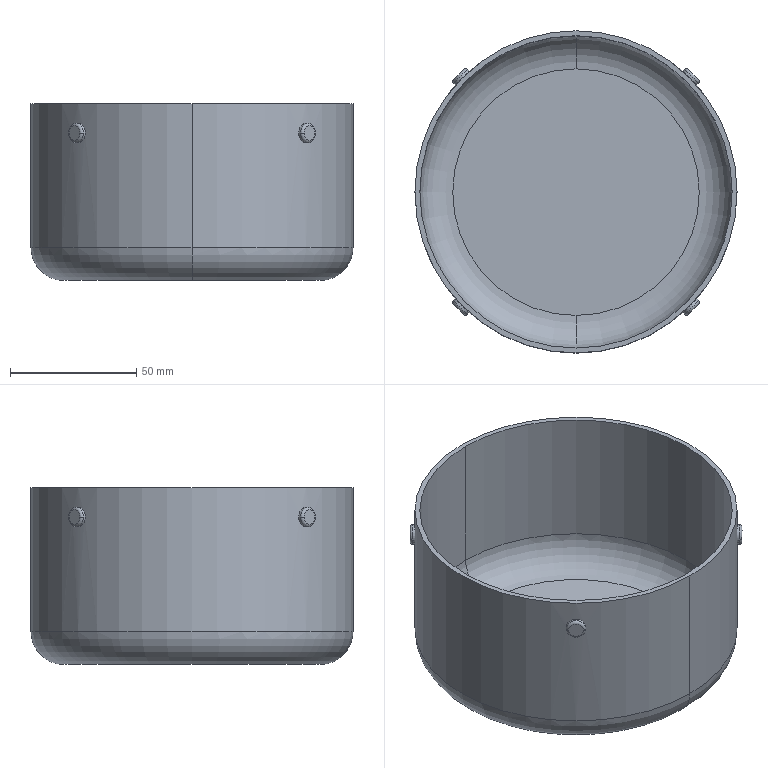Part | NX | features BREP 1 | 1 solid | 115 faces | box 127.4 x 127.4 x 70 mm | volume 77039 mm3 | cylinder 52 | plane 51 | torus 12 | commonest cylinder face diameters 7.8 x8 4.379 x7 5.427 x7 7.616 x7 6.522 x5 3.284 x4